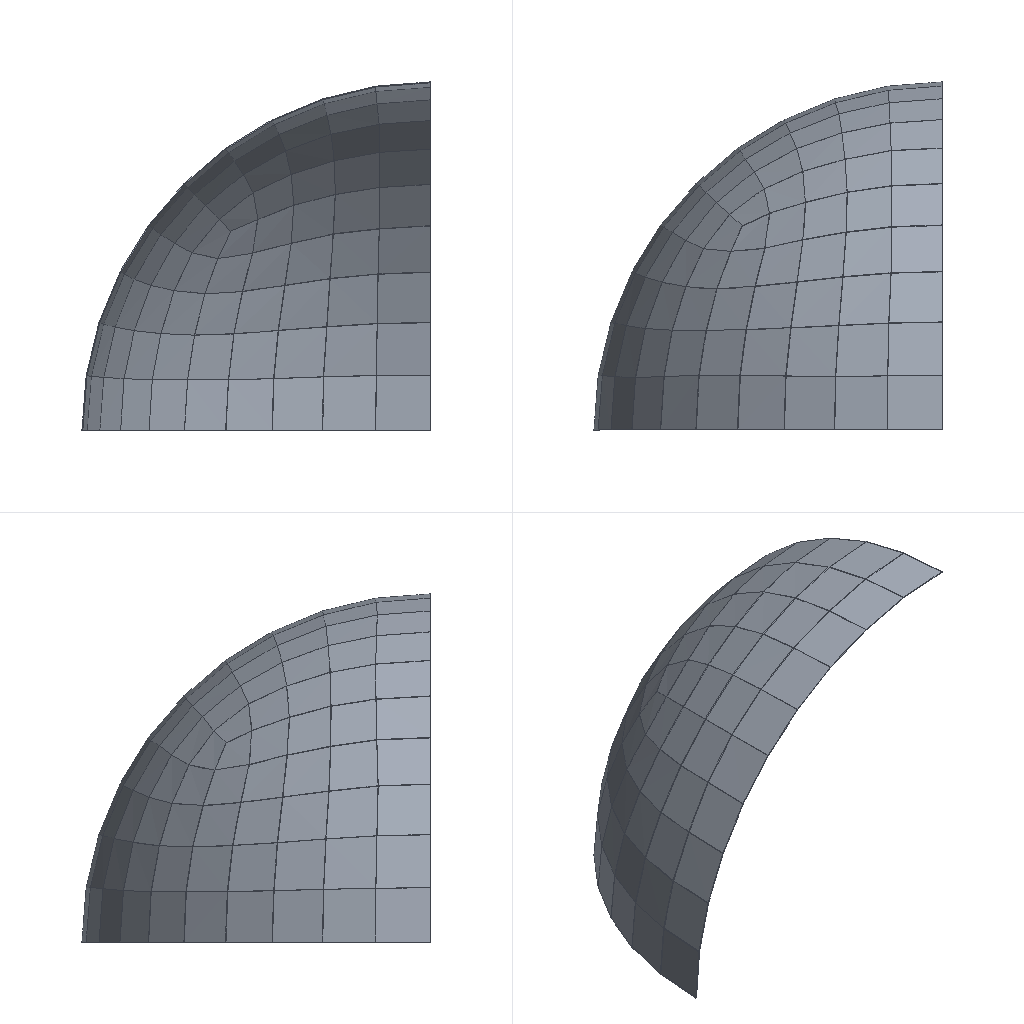Simulation study | ansys workbench
Set-up summary:
category,name,step,type,value,unit,region
solver,ansys_workbench
units,mm-N-s-tonne (MPa),,stated,"/units,MPA"
analysis,LS1,,static
load_step,LS1,LS1,static,nsubst=1; time=1
mesh,nodes,,,603
mesh,elements,,,150
element_type,SOLID186,,,75
element_type,SURF154,,,75
material,Structural Steel,,E,200000,tonne s^-2 mm^-1
material,Structural Steel,,nu,0.3
material,Structural Steel,,density,7.85e-09,tonne mm^-3
material,Structural Steel,,conductivity,60.5,tonne mm s^-3 C^-1
material,Structural Steel,,specific_heat,4.34e+08,mm^2 s^-2 C^-1
material,Structural Steel,,cte,1.2e-05,C^-1
material,Structural Steel,,permeability,10000
material,Structural Steel,,resistivity,0.00017,ohm mm
load,Define Force Using Surface Effect Elements,LS1,surface-effect pres face 3,-20.58,,SURF154 #2
bc,Fixed Supports,model,fixed,[dofs=ALL],,_FIXEDSU
named_set,_FIXEDSU,,node,256
Ansys APDL input file, long lists of numbers shortened:
/batch
/config,noeldb,1     ! force off writing results to database
*get,_wallstrt,active,,time,wall
! ANSYS input file written by Workbench version 2022 R1
! File used for geometry attach:
/title,wbnew--____ (A5)
! ****** Begin Custom Load Command Snippet ******
/COM, ACT Extensions:
/COM,     LSDYNA, 2021.1
/COM,
! ****** End   Custom Load Command Snippet ******
*DIM,_wb_ProjectScratch_dir,string,248
_wb_ProjectScratch_dir(1) = ''
*DIM,_wb_SolverFiles_dir,string,248
_wb_SolverFiles_dir(1) = ''
*DIM,_wb_userfiles_dir,string,248
_wb_userfiles_dir(1) = ''
/com,--- Data in consistent NMM units. See Solving Units in the help system for more information.
/units,MPA
/nopr
/wb,file,start              !  signify a WB generated input file
/prep7
! Turn off shape checking because checks already performed inside WB mesher.
! See help system for more information.
SHPP,OFF,,NOWARN
/nolist
etcon,set             ! allow ANSYS to choose best KEYOP's for 180x elements, resets any applicable keyopt to MAPDL defaults
/com,*********** Nodes for the whole assembly ***********
nblock,3,,663
(1i9,3e20.9e3)
        1    -3.826839856E+00     6.120915030E-01     6.076794252E-01
! (602 more lines like these left out)
-1
/wb,elem,start            !  set before creation of elements
/com,*********** Elements for Body 1 "______-FreeParts|__-__4" ***********
et,1,186
keyo,1,2,1          ! set full integration on SOLID186
eblock,19,solid,,75
(19i9)
        1        1        1        1        0        0        0        0       20        0        1       52       60       61       53       71       63       62       70
! (149 more lines like these left out)
-1
/wb,elem,end               !  done creating elements
/com,*********** Send User Defined Coordinate System(s) ***********
csys,0
toffst,273.15,  ! Temperature offset from absolute zero
/com,*********** Set Reference Temperature ***********
tref,22.
/wb,mat,start              !  starting to send materials
/com,*********** Send Materials ***********
Temperature = 'TEMP' ! Temperature
MP,DENS,1,7.85e-09,	! tonne mm^-3
MP,ALPX,1,1.2e-05,	! C^-1
MP,C,1,434000000,	! mm^2 s^-2 C^-1
MP,KXX,1,60.5,	! tonne mm s^-3 C^-1
MP,RSVX,1,0.00017,	! ohm mm
MP,EX,1,200000,	! tonne s^-2 mm^-1
MP,NUXY,1,0.3,
MP,MURX,1,10000,
/wb,mat,end                !  done sending materials
!************************* Model Summary ********************
!______-FreeParts|__-__4,	结构钢,	matid,	1
!************************* End Model Summary ********************
! get the diagonal of the bounding box. Needed later for other things
*get,_xmin,node,,mnloc,x
*get,_ymin,node,,mnloc,y
*get,_zmin,node,,mnloc,z
*get,_xmax,node,,mxloc,x
*get,_ymax,node,,mxloc,y
*get,_zmax,node,,mxloc,z
_ASMDIAG=(_xmax-_xmin)*(_xmax-_xmin)+(_ymax-_ymin)*(_ymax-_ymin)+(_zmax-_zmin)*(_zmax-_zmin)
_ASMDIAG=SQRT(_ASMDIAG)
/wb,contact,start          !  starting to send contact
/wb,contact,end            !  done creating contacts
/golist
/wb,load,start             !  starting to send loads
/com,*********** Fixed Supports ***********
CMBLOCK,_FIXEDSU,NODE,      256
(8i10)
         1         2         3         4         5         6         7         8
! (31 more lines like these left out)
cmsel,s,_FIXEDSU
d,all,all
nsel,all
/com,*********** Define Force Using Surface Effect Elements ***********
local,12,0,0.,0.,0.,0.,0.,0.
csys,0
et,2,154
eblock,10,,,75
(15i9)
      256        2        2        2       12       62       70       71       63      381      403      384      379
! (74 more lines like these left out)
-1
esel,s,type,,2
keyop,2,2,1                ! Apply load in local coordinate system
keyop,2,7,1                ! Use original area so load is constant in large deformation
esel,all
/gst,on,on
fini
*get,_numnode,node,0,count
*get,_numelem,elem,0,count
*get, _MAXELEMNUM, elem, 0, NUM, MAX
*get, _MAXNODENUM, node, 0, NUM, MAX
*get, _MAXELEMTYPE, etyp, 0, NUM, MAX
*get, _MAXREALCONST, real, 0, NUM, MAX
/go
/wb,load,end               !  done creating loads
/com,--- Number of total nodes = %_numnode%
/com,--- Number of contact elements = 75
/com,--- Number of spring elements = 0
/com,--- Number of bearing elements = 0
/com,--- Number of solid elements = 75
/com,--- Number of condensed parts = 0
/com,--- Number of total elements = %_numelem%
*get,_wallbsol,active,,time,wall
/com,****************************************************************************
/com,*************************    SOLUTION       ********************************
/com,****************************************************************************
/solu
antype,0                   ! static analysis
_thickRatio=  0     ! Ratio of thick parts in the model
eqsl,sparse,,,,,1
cntr,print,1               ! print out contact info and also make no initial contact an error
dmpoption,emat,no             ! Don't combine emat file for DANSYS
dmpoption,esav,no             ! Don't combine esav file for DANSYS
nldiag,cont,iter           ! print out contact info each equilibrium iteration
rescontrol,,none                 ! Do not keep any restart files
/com,****************************************************
/com,******************* SOLVE FOR LS 1 OF 1 ****************
esel,s,type,,2
nsle
sfe,all,1,pres,1,0.
sfe,all,2,pres,1,0.
sfe,all,3,pres,1,-20.58
nsel,all
esel,all
/nopr
/gopr
nsub,1,1,1
time,1.
outres,erase
outres,all,none
outres,nsol,all,
outres,rsol,all
outres,eangl,all
outres,etmp,all
outres,veng,all
outres,strs,all,
outres,epel,all,
outres,eppl,all,
outres,cont,all,
! *********** WB SOLVE COMMAND ***********
! check interactive state
*get,ANSINTER_,active,,int
*if,ANSINTER_,ne,0,then
/eof
*endif
solve
/com *************** Write FE CONNECTORS *********
CEWRITE,file,ce,,INTE
/com,****************************************************
/com,*************** FINISHED SOLVE FOR LS 1 *************
*get,_wallasol,active,,time,wall
/nopr
*get,_numnode,node,0,count
*get,_numelem,elem,0,count
*get, _MAXELEMNUM, elem, 0, NUM, MAX
*get, _MAXNODENUM, node, 0, NUM, MAX,,,INTERNAL
*get, _MAXELEMTYPE, etyp, 0, NUM, MAX
*get, _MAXREALCONST, real, 0, NUM, MAX
/gopr
/post1
xmlo,ENCODING,ISO-8859-1
xmlo,parm
/xml,parm,xml
fini
/gopr
*get,_walldone,active,,time,wall
_preptime=(_wallbsol-_wallstrt)*3600
_solvtime=(_wallasol-_wallbsol)*3600
_posttime=(_walldone-_wallasol)*3600
_totaltim=(_walldone-_wallstrt)*3600
*get,_dlbratio,active,0,solu,dlbr
*get,_combtime,active,0,solu,comb
*get,_ssmode,active,0,solu,ssmm
*get,_ndofs,active,0,solu,ndof
*get,_sol_end_time,active,0,set,time
*if,_sol_end_time,eq,1.,then
/fclean				!clean distributed files
*endif
/com,--- Total number of nodes = %_numnode%
/com,--- Total number of elements = %_numelem%
/com,--- Element load balance ratio = %_dlbratio%
/com,--- Time to combine distributed files = %_combtime%
/com,--- Sparse memory mode = %_ssmode%
/com,--- Number of DOF = %_ndofs%
/wb,file,end               ! done with WB generated input
Results summary:
result,analyses[0].index,,,1
result,analyses[0].system,,,SYS
result,analyses[0].deck,,,deck.dat
result,analyses[0].solve_status,,,completed
result,analyses[0].analysis_type,,,static
result,analyses[0].physics,,,mechanical
result,analyses[0].unit_system,,,"NMM: mm, ton, N, s, mV, mA, degC"
result,analyses[0].n_sets,,,1
result,analyses[0].load_steps[0].set,set=1,,1
result,analyses[0].load_steps[0].time_or_freq,set=1,,1
result,analyses[0].load_steps[0].max_displacement_magnitude,set=1,,5.09084e-06
result,analyses[0].load_steps[0].max_von_mises_nodal,set=1,,36.993
result,analyses[0].load_steps[0].reaction_force_sum_xyz[1],set=1,,-4.28433e-14
result,analyses[0].load_steps[0].reaction_force_sum_xyz[2],set=1,,-1.36176e-14
result,analyses[0].load_steps[0].reaction_force_sum_xyz[3],set=1,,500